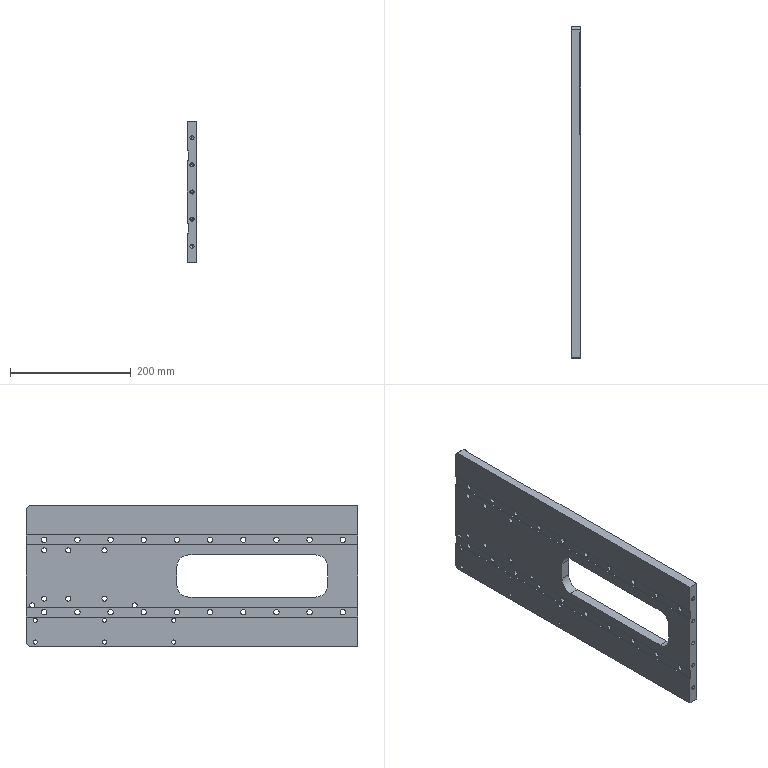Part | SolidWorks | features HoleWzd 5, ICE 4, Chamfer 1, Extrusion 1, Fillet 1, LPattern 1 | 1 solid | 186 faces | box 16 x 550 x 235 mm | volume 1648146 mm3 | cylinder 126 | plane 46 | cone 14 | commonest cylinder face diameters 9 x40 15 x40 6.8 x22 8.5 x12 8 x4 10 x4